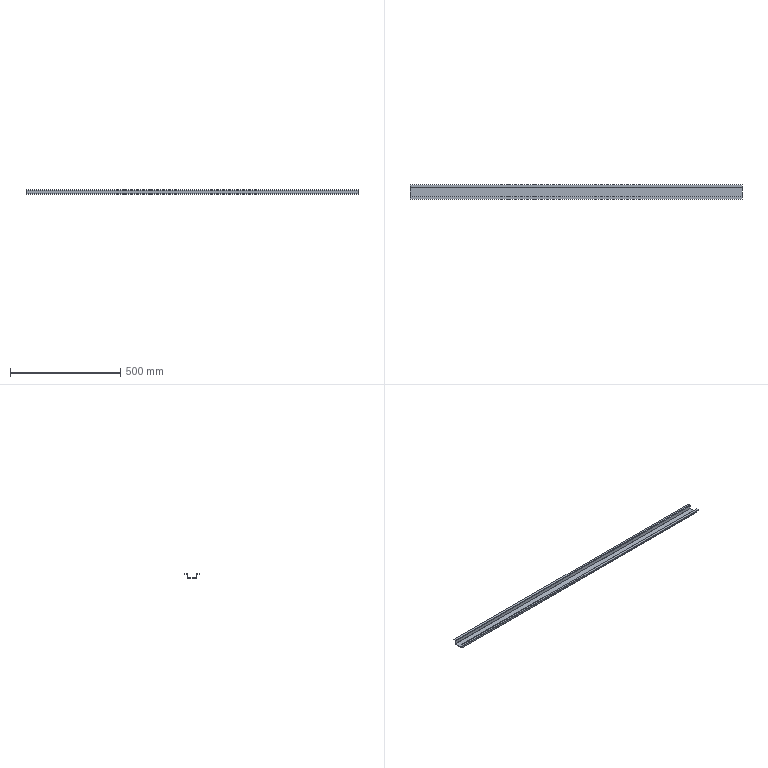Part | SolidWorks | features BaseBody 1 | 1 solid | 22 faces | box 1507 x 64 x 20 mm | volume 295191 mm3 | plane 14 | cylinder 8 | commonest cylinder face diameters 0.4 x4 4.4 x4
STEP:
#1=CARTESIAN_POINT('',(-730.,-22.2,-4.));
#2=VERTEX_POINT('',#1);
#3=CARTESIAN_POINT('',(-730.,-22.,-4.2));
#4=VERTEX_POINT('',#3);
#5=CARTESIAN_POINT('',(-730.,-22.2,-4.2));
#6=DIRECTION('',(-1.,0.,0.));
#7=DIRECTION('',(0.,0.,1.));
#8=AXIS2_PLACEMENT_3D('',#5,#6,#7);
#9=CIRCLE('',#8,0.2);
#10=EDGE_CURVE('',#2,#4,#9,.T.);
#11=ORIENTED_EDGE('',*,*,#10,.T.);
#12=CARTESIAN_POINT('',(777.,-22.,-4.2));
#13=VERTEX_POINT('',#12);
#14=CARTESIAN_POINT('',(777.,-22.,-4.2));
#15=DIRECTION('',(-1.,0.,0.));
#16=VECTOR('',#15,1000.);
#17=LINE('',#14,#16);
#18=EDGE_CURVE('',#13,#4,#17,.T.);
#19=ORIENTED_EDGE('',*,*,#18,.F.);
#20=CARTESIAN_POINT('',(777.,-22.2,-4.));
#21=VERTEX_POINT('',#20);
#22=CARTESIAN_POINT('',(777.,-22.2,-4.2));
#23=DIRECTION('',(1.,0.,0.));
#24=DIRECTION('',(0.,0.,1.));
#25=AXIS2_PLACEMENT_3D('',#22,#23,#24);
#26=CIRCLE('',#25,0.2);
#27=EDGE_CURVE('',#13,#21,#26,.T.);
#28=ORIENTED_EDGE('',*,*,#27,.T.);
#29=CARTESIAN_POINT('',(777.,-22.2,-4.));
#30=DIRECTION('',(1.,0.,0.));
#31=VECTOR('',#30,1000.);
#32=LINE('',#29,#31);
#33=EDGE_CURVE('',#2,#21,#32,.T.);
#34=ORIENTED_EDGE('',*,*,#33,.F.);
#35=EDGE_LOOP('',(#11,#19,#28,#34));
#36=FACE_OUTER_BOUND('',#35,.T.);
#37=CARTESIAN_POINT('',(2285.24,-22.2,-4.2));
#38=DIRECTION('',(-1.,0.,0.));
#39=DIRECTION('',(0.,0.,1.));
#40=AXIS2_PLACEMENT_3D('',#37,#38,#39);
#41=CYLINDRICAL_SURFACE('',#40,0.2);
#42=ADVANCED_FACE('',(#36),#41,.F.);
#43=CARTESIAN_POINT('',(-730.,-22.2,-2.));
#44=VERTEX_POINT('',#43);
#45=CARTESIAN_POINT('',(-730.,-20.,-4.2));
#46=VERTEX_POINT('',#45);
#47=CARTESIAN_POINT('',(-730.,-22.2,-4.2));
#48=DIRECTION('',(-1.,0.,0.));
#49=DIRECTION('',(0.,0.,1.));
#50=AXIS2_PLACEMENT_3D('',#47,#48,#49);
#51=CIRCLE('',#50,2.2);
#52=EDGE_CURVE('',#44,#46,#51,.T.);
#53=ORIENTED_EDGE('',*,*,#52,.F.);
#54=CARTESIAN_POINT('',(777.,-22.2,-2.));
#55=VERTEX_POINT('',#54);
#56=CARTESIAN_POINT('',(777.,-22.2,-2.));
#57=DIRECTION('',(1.,0.,0.));
#58=VECTOR('',#57,1000.);
#59=LINE('',#56,#58);
#60=EDGE_CURVE('',#44,#55,#59,.T.);
#61=ORIENTED_EDGE('',*,*,#60,.T.);
#62=CARTESIAN_POINT('',(777.,-20.,-4.2));
#63=VERTEX_POINT('',#62);
#64=CARTESIAN_POINT('',(777.,-22.2,-4.2));
#65=DIRECTION('',(1.,0.,0.));
#66=DIRECTION('',(0.,0.,1.));
#67=AXIS2_PLACEMENT_3D('',#64,#65,#66);
#68=CIRCLE('',#67,2.2);
#69=EDGE_CURVE('',#63,#55,#68,.T.);
#70=ORIENTED_EDGE('',*,*,#69,.F.);
#71=CARTESIAN_POINT('',(777.,-20.,-4.2));
#72=DIRECTION('',(-1.,0.,0.));
#73=VECTOR('',#72,1000.);
#74=LINE('',#71,#73);
#75=EDGE_CURVE('',#63,#46,#74,.T.);
#76=ORIENTED_EDGE('',*,*,#75,.T.);
#77=EDGE_LOOP('',(#53,#61,#70,#76));
#78=FACE_OUTER_BOUND('',#77,.T.);
#79=CARTESIAN_POINT('',(2285.24,-22.2,-4.2));
#80=DIRECTION('',(-1.,0.,0.));
#81=DIRECTION('',(0.,0.,1.));
#82=AXIS2_PLACEMENT_3D('',#79,#80,#81);
#83=CYLINDRICAL_SURFACE('',#82,2.2);
#84=ADVANCED_FACE('',(#78),#83,.T.);
#85=CARTESIAN_POINT('',(777.,22.2,-4.));
#86=VERTEX_POINT('',#85);
#87=CARTESIAN_POINT('',(777.,22.,-4.2));
#88=VERTEX_POINT('',#87);
#89=CARTESIAN_POINT('',(777.,22.2,-4.2));
#90=DIRECTION('',(1.,0.,0.));
#91=DIRECTION('',(0.,0.,-1.));
#92=AXIS2_PLACEMENT_3D('',#89,#90,#91);
#93=CIRCLE('',#92,0.2);
#94=EDGE_CURVE('',#86,#88,#93,.T.);
#95=ORIENTED_EDGE('',*,*,#94,.T.);
#96=CARTESIAN_POINT('',(-730.,22.,-4.2));
#97=VERTEX_POINT('',#96);
#98=CARTESIAN_POINT('',(-730.,22.,-4.2));
#99=DIRECTION('',(1.,0.,0.));
#100=VECTOR('',#99,1000.);
#101=LINE('',#98,#100);
#102=EDGE_CURVE('',#97,#88,#101,.T.);
#103=ORIENTED_EDGE('',*,*,#102,.F.);
#104=CARTESIAN_POINT('',(-730.,22.2,-4.));
#105=VERTEX_POINT('',#104);
#106=CARTESIAN_POINT('',(-730.,22.2,-4.2));
#107=DIRECTION('',(-1.,0.,0.));
#108=DIRECTION('',(0.,0.,-1.));
#109=AXIS2_PLACEMENT_3D('',#106,#107,#108);
#110=CIRCLE('',#109,0.2);
#111=EDGE_CURVE('',#97,#105,#110,.T.);
#112=ORIENTED_EDGE('',*,*,#111,.T.);
#113=CARTESIAN_POINT('',(-730.,22.2,-4.));
#114=DIRECTION('',(-1.,0.,0.));
#115=VECTOR('',#114,1000.);
#116=LINE('',#113,#115);
#117=EDGE_CURVE('',#86,#105,#116,.T.);
#118=ORIENTED_EDGE('',*,*,#117,.F.);
#119=EDGE_LOOP('',(#95,#103,#112,#118));
#120=FACE_OUTER_BOUND('',#119,.T.);
#121=CARTESIAN_POINT('',(-2237.915,22.2,-4.2));
#122=DIRECTION('',(1.,0.,0.));
#123=DIRECTION('',(0.,0.,-1.));
#124=AXIS2_PLACEMENT_3D('',#121,#122,#123);
#125=CYLINDRICAL_SURFACE('',#124,0.2);
#126=ADVANCED_FACE('',(#120),#125,.F.);
#127=CARTESIAN_POINT('',(777.,22.2,-2.));
#128=VERTEX_POINT('',#127);
#129=CARTESIAN_POINT('',(777.,20.,-4.2));
#130=VERTEX_POINT('',#129);
#131=CARTESIAN_POINT('',(777.,22.2,-4.2));
#132=DIRECTION('',(1.,0.,0.));
#133=DIRECTION('',(0.,0.,-1.));
#134=AXIS2_PLACEMENT_3D('',#131,#132,#133);
#135=CIRCLE('',#134,2.2);
#136=EDGE_CURVE('',#128,#130,#135,.T.);
#137=ORIENTED_EDGE('',*,*,#136,.F.);
#138=CARTESIAN_POINT('',(-730.,22.2,-2.));
#139=VERTEX_POINT('',#138);
#140=CARTESIAN_POINT('',(-730.,22.2,-2.));
#141=DIRECTION('',(-1.,0.,0.));
#142=VECTOR('',#141,1000.);
#143=LINE('',#140,#142);
#144=EDGE_CURVE('',#128,#139,#143,.T.);
#145=ORIENTED_EDGE('',*,*,#144,.T.);
#146=CARTESIAN_POINT('',(-730.,20.,-4.2));
#147=VERTEX_POINT('',#146);
#148=CARTESIAN_POINT('',(-730.,22.2,-4.2));
#149=DIRECTION('',(-1.,0.,0.));
#150=DIRECTION('',(0.,0.,-1.));
#151=AXIS2_PLACEMENT_3D('',#148,#149,#150);
#152=CIRCLE('',#151,2.2);
#153=EDGE_CURVE('',#147,#139,#152,.T.);
#154=ORIENTED_EDGE('',*,*,#153,.F.);
#155=CARTESIAN_POINT('',(-730.,20.,-4.2));
#156=DIRECTION('',(1.,0.,0.));
#157=VECTOR('',#156,1000.);
#158=LINE('',#155,#157);
#159=EDGE_CURVE('',#147,#130,#158,.T.);
#160=ORIENTED_EDGE('',*,*,#159,.T.);
#161=EDGE_LOOP('',(#137,#145,#154,#160));
#162=FACE_OUTER_BOUND('',#161,.T.);
#163=CARTESIAN_POINT('',(-2237.915,22.2,-4.2));
#164=DIRECTION('',(1.,0.,0.));
#165=DIRECTION('',(0.,0.,-1.));
#166=AXIS2_PLACEMENT_3D('',#163,#164,#165);
#167=CYLINDRICAL_SURFACE('',#166,2.2);
#168=ADVANCED_FACE('',(#162),#167,.T.);
#169=CARTESIAN_POINT('',(777.,20.,-19.8));
#170=VERTEX_POINT('',#169);
#171=CARTESIAN_POINT('',(777.,19.8,-20.));
#172=VERTEX_POINT('',#171);
#173=CARTESIAN_POINT('',(777.,19.8,-19.8));
#174=DIRECTION('',(-1.,0.,0.));
#175=DIRECTION('',(0.,0.,1.));
#176=AXIS2_PLACEMENT_3D('',#173,#174,#175);
#177=CIRCLE('',#176,0.2);
#178=EDGE_CURVE('',#170,#172,#177,.T.);
#179=ORIENTED_EDGE('',*,*,#178,.F.);
#180=CARTESIAN_POINT('',(-730.,20.,-19.8));
#181=VERTEX_POINT('',#180);
#182=CARTESIAN_POINT('',(777.,20.,-19.8));
#183=DIRECTION('',(-1.,0.,0.));
#184=VECTOR('',#183,1000.);
#185=LINE('',#182,#184);
#186=EDGE_CURVE('',#170,#181,#185,.T.);
#187=ORIENTED_EDGE('',*,*,#186,.T.);
#188=CARTESIAN_POINT('',(-730.,19.8,-20.));
#189=VERTEX_POINT('',#188);
#190=CARTESIAN_POINT('',(-730.,19.8,-19.8));
#191=DIRECTION('',(1.,0.,0.));
#192=DIRECTION('',(0.,0.,1.));
#193=AXIS2_PLACEMENT_3D('',#190,#191,#192);
#194=CIRCLE('',#193,0.2);
#195=EDGE_CURVE('',#189,#181,#194,.T.);
#196=ORIENTED_EDGE('',*,*,#195,.F.);
#197=CARTESIAN_POINT('',(777.,19.8,-20.));
#198=DIRECTION('',(-1.,0.,0.));
#199=VECTOR('',#198,1000.);
#200=LINE('',#197,#199);
#201=EDGE_CURVE('',#172,#189,#200,.T.);
#202=ORIENTED_EDGE('',*,*,#201,.F.);
#203=EDGE_LOOP('',(#179,#187,#196,#202));
#204=FACE_OUTER_BOUND('',#203,.T.);
#205=CARTESIAN_POINT('',(2285.87,19.8,-19.8));
#206=DIRECTION('',(-1.,0.,0.));
#207=DIRECTION('',(0.,0.,1.));
#208=AXIS2_PLACEMENT_3D('',#205,#206,#207);
#209=CYLINDRICAL_SURFACE('',#208,0.2);
#210=ADVANCED_FACE('',(#204),#209,.F.);
#211=CARTESIAN_POINT('',(777.,22.,-19.8));
#212=VERTEX_POINT('',#211);
#213=CARTESIAN_POINT('',(777.,19.8,-22.));
#214=VERTEX_POINT('',#213);
#215=CARTESIAN_POINT('',(777.,19.8,-19.8));
#216=DIRECTION('',(-1.,0.,0.));
#217=DIRECTION('',(0.,0.,1.));
#218=AXIS2_PLACEMENT_3D('',#215,#216,#217);
#219=CIRCLE('',#218,2.2);
#220=EDGE_CURVE('',#212,#214,#219,.T.);
#221=ORIENTED_EDGE('',*,*,#220,.T.);
#222=CARTESIAN_POINT('',(-730.,19.8,-22.));
#223=VERTEX_POINT('',#222);
#224=CARTESIAN_POINT('',(777.,19.8,-22.));
#225=DIRECTION('',(-1.,0.,0.));
#226=VECTOR('',#225,1000.);
#227=LINE('',#224,#226);
#228=EDGE_CURVE('',#214,#223,#227,.T.);
#229=ORIENTED_EDGE('',*,*,#228,.T.);
#230=CARTESIAN_POINT('',(-730.,22.,-19.8));
#231=VERTEX_POINT('',#230);
#232=CARTESIAN_POINT('',(-730.,19.8,-19.8));
#233=DIRECTION('',(1.,0.,0.));
#234=DIRECTION('',(0.,0.,1.));
#235=AXIS2_PLACEMENT_3D('',#232,#233,#234);
#236=CIRCLE('',#235,2.2);
#237=EDGE_CURVE('',#223,#231,#236,.T.);
#238=ORIENTED_EDGE('',*,*,#237,.T.);
#239=CARTESIAN_POINT('',(777.,22.,-19.8));
#240=DIRECTION('',(-1.,0.,0.));
#241=VECTOR('',#240,1000.);
#242=LINE('',#239,#241);
#243=EDGE_CURVE('',#212,#231,#242,.T.);
#244=ORIENTED_EDGE('',*,*,#243,.F.);
#245=EDGE_LOOP('',(#221,#229,#238,#244));
#246=FACE_OUTER_BOUND('',#245,.T.);
#247=CARTESIAN_POINT('',(2285.87,19.8,-19.8));
#248=DIRECTION('',(-1.,0.,0.));
#249=DIRECTION('',(0.,0.,1.));
#250=AXIS2_PLACEMENT_3D('',#247,#248,#249);
#251=CYLINDRICAL_SURFACE('',#250,2.2);
#252=ADVANCED_FACE('',(#246),#251,.T.);
#253=CARTESIAN_POINT('',(-730.,-20.,-19.8));
#254=VERTEX_POINT('',#253);
#255=CARTESIAN_POINT('',(-730.,-19.8,-20.));
#256=VERTEX_POINT('',#255);
#257=CARTESIAN_POINT('',(-730.,-19.8,-19.8));
#258=DIRECTION('',(1.,0.,0.));
#259=DIRECTION('',(0.,0.,-1.));
#260=AXIS2_PLACEMENT_3D('',#257,#258,#259);
#261=CIRCLE('',#260,0.2);
#262=EDGE_CURVE('',#254,#256,#261,.T.);
#263=ORIENTED_EDGE('',*,*,#262,.F.);
#264=CARTESIAN_POINT('',(777.,-20.,-19.8));
#265=VERTEX_POINT('',#264);
#266=CARTESIAN_POINT('',(-730.,-20.,-19.8));
#267=DIRECTION('',(1.,0.,0.));
#268=VECTOR('',#267,1000.);
#269=LINE('',#266,#268);
#270=EDGE_CURVE('',#254,#265,#269,.T.);
#271=ORIENTED_EDGE('',*,*,#270,.T.);
#272=CARTESIAN_POINT('',(777.,-19.8,-20.));
#273=VERTEX_POINT('',#272);
#274=CARTESIAN_POINT('',(777.,-19.8,-19.8));
#275=DIRECTION('',(-1.,0.,0.));
#276=DIRECTION('',(0.,0.,-1.));
#277=AXIS2_PLACEMENT_3D('',#274,#275,#276);
#278=CIRCLE('',#277,0.2);
#279=EDGE_CURVE('',#273,#265,#278,.T.);
#280=ORIENTED_EDGE('',*,*,#279,.F.);
#281=CARTESIAN_POINT('',(-730.,-19.8,-20.));
#282=DIRECTION('',(1.,0.,0.));
#283=VECTOR('',#282,1000.);
#284=LINE('',#281,#283);
#285=EDGE_CURVE('',#256,#273,#284,.T.);
#286=ORIENTED_EDGE('',*,*,#285,.F.);
#287=EDGE_LOOP('',(#263,#271,#280,#286));
#288=FACE_OUTER_BOUND('',#287,.T.);
#289=CARTESIAN_POINT('',(-2239.98,-19.8,-19.8));
#290=DIRECTION('',(1.,0.,0.));
#291=DIRECTION('',(0.,0.,-1.));
#292=AXIS2_PLACEMENT_3D('',#289,#290,#291);
#293=CYLINDRICAL_SURFACE('',#292,0.2);
#294=ADVANCED_FACE('',(#288),#293,.F.);
#295=CARTESIAN_POINT('',(-730.,-22.,-19.8));
#296=VERTEX_POINT('',#295);
#297=CARTESIAN_POINT('',(-730.,-19.8,-22.));
#298=VERTEX_POINT('',#297);
#299=CARTESIAN_POINT('',(-730.,-19.8,-19.8));
#300=DIRECTION('',(1.,0.,0.));
#301=DIRECTION('',(0.,0.,-1.));
#302=AXIS2_PLACEMENT_3D('',#299,#300,#301);
#303=CIRCLE('',#302,2.2);
#304=EDGE_CURVE('',#296,#298,#303,.T.);
#305=ORIENTED_EDGE('',*,*,#304,.T.);
#306=CARTESIAN_POINT('',(777.,-19.8,-22.));
#307=VERTEX_POINT('',#306);
#308=CARTESIAN_POINT('',(-730.,-19.8,-22.));
#309=DIRECTION('',(1.,0.,0.));
#310=VECTOR('',#309,1000.);
#311=LINE('',#308,#310);
#312=EDGE_CURVE('',#298,#307,#311,.T.);
#313=ORIENTED_EDGE('',*,*,#312,.T.);
#314=CARTESIAN_POINT('',(777.,-22.,-19.8));
#315=VERTEX_POINT('',#314);
#316=CARTESIAN_POINT('',(777.,-19.8,-19.8));
#317=DIRECTION('',(-1.,0.,0.));
#318=DIRECTION('',(0.,0.,-1.));
#319=AXIS2_PLACEMENT_3D('',#316,#317,#318);
#320=CIRCLE('',#319,2.2);
#321=EDGE_CURVE('',#307,#315,#320,.T.);
#322=ORIENTED_EDGE('',*,*,#321,.T.);
#323=CARTESIAN_POINT('',(-730.,-22.,-19.8));
#324=DIRECTION('',(1.,0.,0.));
#325=VECTOR('',#324,1000.);
#326=LINE('',#323,#325);
#327=EDGE_CURVE('',#296,#315,#326,.T.);
#328=ORIENTED_EDGE('',*,*,#327,.F.);
#329=EDGE_LOOP('',(#305,#313,#322,#328));
#330=FACE_OUTER_BOUND('',#329,.T.);
#331=CARTESIAN_POINT('',(-2239.98,-19.8,-19.8));
#332=DIRECTION('',(1.,0.,0.));
#333=DIRECTION('',(0.,0.,-1.));
#334=AXIS2_PLACEMENT_3D('',#331,#332,#333);
#335=CYLINDRICAL_SURFACE('',#334,2.2);
#336=ADVANCED_FACE('',(#330),#335,.T.);
#337=ORIENTED_EDGE('',*,*,#228,.F.);
#338=CARTESIAN_POINT('',(777.,20.,-22.));
#339=DIRECTION('',(0.,-1.,0.));
#340=VECTOR('',#339,1000.);
#341=LINE('',#338,#340);
#342=EDGE_CURVE('',#214,#307,#341,.T.);
#343=ORIENTED_EDGE('',*,*,#342,.T.);
#344=ORIENTED_EDGE('',*,*,#312,.F.);
#345=CARTESIAN_POINT('',(-730.,20.,-22.));
#346=DIRECTION('',(0.,-1.,0.));
#347=VECTOR('',#346,1000.);
#348=LINE('',#345,#347);
#349=EDGE_CURVE('',#223,#298,#348,.T.);
#350=ORIENTED_EDGE('',*,*,#349,.F.);
#351=EDGE_LOOP('',(#337,#343,#344,#350));
#352=FACE_OUTER_BOUND('',#351,.T.);
#353=CARTESIAN_POINT('',(-740.,20.,-22.));
#354=DIRECTION('',(0.,0.,1.));
#355=DIRECTION('',(1.,0.,0.));
#356=AXIS2_PLACEMENT_3D('',#353,#354,#355);
#357=PLANE('',#356);
#358=ADVANCED_FACE('',(#352),#357,.F.);
#359=CARTESIAN_POINT('',(777.,20.,-20.));
#360=DIRECTION('',(0.,-1.,0.));
#361=VECTOR('',#360,1000.);
#362=LINE('',#359,#361);
#363=EDGE_CURVE('',#172,#273,#362,.T.);
#364=ORIENTED_EDGE('',*,*,#363,.F.);
#365=ORIENTED_EDGE('',*,*,#201,.T.);
#366=CARTESIAN_POINT('',(-730.,20.,-20.));
#367=DIRECTION('',(0.,-1.,0.));
#368=VECTOR('',#367,1000.);
#369=LINE('',#366,#368);
#370=EDGE_CURVE('',#189,#256,#369,.T.);
#371=ORIENTED_EDGE('',*,*,#370,.T.);
#372=ORIENTED_EDGE('',*,*,#285,.T.);
#373=EDGE_LOOP('',(#364,#365,#371,#372));
#374=FACE_OUTER_BOUND('',#373,.T.);
#375=CARTESIAN_POINT('',(-740.,20.,-20.));
#376=DIRECTION('',(0.,0.,1.));
#377=DIRECTION('',(1.,0.,0.));
#378=AXIS2_PLACEMENT_3D('',#375,#376,#377);
#379=PLANE('',#378);
#380=ADVANCED_FACE('',(#374),#379,.T.);
#381=ORIENTED_EDGE('',*,*,#75,.F.);
#382=CARTESIAN_POINT('',(777.,-20.,-20.));
#383=DIRECTION('',(0.,0.,1.));
#384=VECTOR('',#383,1000.);
#385=LINE('',#382,#384);
#386=EDGE_CURVE('',#265,#63,#385,.T.);
#387=ORIENTED_EDGE('',*,*,#386,.F.);
#388=ORIENTED_EDGE('',*,*,#270,.F.);
#389=CARTESIAN_POINT('',(-730.,-20.,-20.));
#390=DIRECTION('',(0.,0.,1.));
#391=VECTOR('',#390,1000.);
#392=LINE('',#389,#391);
#393=EDGE_CURVE('',#254,#46,#392,.T.);
#394=ORIENTED_EDGE('',*,*,#393,.T.);
#395=EDGE_LOOP('',(#381,#387,#388,#394));
#396=FACE_OUTER_BOUND('',#395,.T.);
#397=CARTESIAN_POINT('',(-740.,-20.,-20.));
#398=DIRECTION('',(0.,1.,0.));
#399=DIRECTION('',(0.,0.,-1.));
#400=AXIS2_PLACEMENT_3D('',#397,#398,#399);
#401=PLANE('',#400);
#402=ADVANCED_FACE('',(#396),#401,.T.);
#403=CARTESIAN_POINT('',(777.,-22.,-20.));
#404=DIRECTION('',(0.,0.,1.));
#405=VECTOR('',#404,1000.);
#406=LINE('',#403,#405);
#407=EDGE_CURVE('',#315,#13,#406,.T.);
#408=ORIENTED_EDGE('',*,*,#407,.T.);
#409=ORIENTED_EDGE('',*,*,#18,.T.);
#410=CARTESIAN_POINT('',(-730.,-22.,-20.));
#411=DIRECTION('',(0.,0.,1.));
#412=VECTOR('',#411,1000.);
#413=LINE('',#410,#412);
#414=EDGE_CURVE('',#296,#4,#413,.T.);
#415=ORIENTED_EDGE('',*,*,#414,.F.);
#416=ORIENTED_EDGE('',*,*,#327,.T.);
#417=EDGE_LOOP('',(#408,#409,#415,#416));
#418=FACE_OUTER_BOUND('',#417,.T.);
#419=CARTESIAN_POINT('',(-740.,-22.,-20.));
#420=DIRECTION('',(0.,1.,0.));
#421=DIRECTION('',(0.,0.,-1.));
#422=AXIS2_PLACEMENT_3D('',#419,#420,#421);
#423=PLANE('',#422);
#424=ADVANCED_FACE('',(#418),#423,.F.);
#425=ORIENTED_EDGE('',*,*,#159,.F.);
#426=CARTESIAN_POINT('',(-730.,20.,-20.));
#427=DIRECTION('',(0.,0.,-1.));
#428=VECTOR('',#427,1000.);
#429=LINE('',#426,#428);
#430=EDGE_CURVE('',#147,#181,#429,.T.);
#431=ORIENTED_EDGE('',*,*,#430,.T.);
#432=ORIENTED_EDGE('',*,*,#186,.F.);
#433=CARTESIAN_POINT('',(777.,20.,-20.));
#434=DIRECTION('',(0.,0.,-1.));
#435=VECTOR('',#434,1000.);
#436=LINE('',#433,#435);
#437=EDGE_CURVE('',#130,#170,#436,.T.);
#438=ORIENTED_EDGE('',*,*,#437,.F.);
#439=EDGE_LOOP('',(#425,#431,#432,#438));
#440=FACE_OUTER_BOUND('',#439,.T.);
#441=CARTESIAN_POINT('',(-740.,20.,-20.));
#442=DIRECTION('',(0.,-1.,0.));
#443=DIRECTION('',(-1.,0.,0.));
#444=AXIS2_PLACEMENT_3D('',#441,#442,#443);
#445=PLANE('',#444);
#446=ADVANCED_FACE('',(#440),#445,.T.);
#447=CARTESIAN_POINT('',(-730.,22.,-20.));
#448=DIRECTION('',(0.,0.,-1.));
#449=VECTOR('',#448,1000.);
#450=LINE('',#447,#449);
#451=EDGE_CURVE('',#97,#231,#450,.T.);
#452=ORIENTED_EDGE('',*,*,#451,.F.);
#453=ORIENTED_EDGE('',*,*,#102,.T.);
#454=CARTESIAN_POINT('',(777.,22.,-20.));
#455=DIRECTION('',(0.,0.,-1.));
#456=VECTOR('',#455,1000.);
#457=LINE('',#454,#456);
#458=EDGE_CURVE('',#88,#212,#457,.T.);
#459=ORIENTED_EDGE('',*,*,#458,.T.);
#460=ORIENTED_EDGE('',*,*,#243,.T.);
#461=EDGE_LOOP('',(#452,#453,#459,#460));
#462=FACE_OUTER_BOUND('',#461,.T.);
#463=CARTESIAN_POINT('',(-740.,22.,-20.));
#464=DIRECTION('',(0.,-1.,0.));
#465=DIRECTION('',(-1.,0.,0.));
#466=AXIS2_PLACEMENT_3D('',#463,#464,#465);
#467=PLANE('',#466);
#468=ADVANCED_FACE('',(#462),#467,.F.);
#469=CARTESIAN_POINT('',(777.,32.,-4.));
#470=VERTEX_POINT('',#469);
#471=CARTESIAN_POINT('',(777.,20.,-4.));
#472=DIRECTION('',(0.,-1.,0.));
#473=VECTOR('',#472,1000.);
#474=LINE('',#471,#473);
#475=EDGE_CURVE('',#470,#86,#474,.T.);
#476=ORIENTED_EDGE('',*,*,#475,.T.);
#477=ORIENTED_EDGE('',*,*,#117,.T.);
#478=CARTESIAN_POINT('',(-730.,32.,-4.));
#479=VERTEX_POINT('',#478);
#480=CARTESIAN_POINT('',(-730.,20.,-4.));
#481=DIRECTION('',(0.,-1.,0.));
#482=VECTOR('',#481,1000.);
#483=LINE('',#480,#482);
#484=EDGE_CURVE('',#479,#105,#483,.T.);
#485=ORIENTED_EDGE('',*,*,#484,.F.);
#486=CARTESIAN_POINT('',(-740.,32.,-4.));
#487=DIRECTION('',(1.,0.,0.));
#488=VECTOR('',#487,1000.);
#489=LINE('',#486,#488);
#490=EDGE_CURVE('',#479,#470,#489,.T.);
#491=ORIENTED_EDGE('',*,*,#490,.T.);
#492=EDGE_LOOP('',(#476,#477,#485,#491));
#493=FACE_OUTER_BOUND('',#492,.T.);
#494=CARTESIAN_POINT('',(-740.,20.,-4.));
#495=DIRECTION('',(0.,0.,1.));
#496=DIRECTION('',(1.,0.,0.));
#497=AXIS2_PLACEMENT_3D('',#494,#495,#496);
#498=PLANE('',#497);
#499=ADVANCED_FACE('',(#493),#498,.F.);
#500=ORIENTED_EDGE('',*,*,#144,.F.);
#501=CARTESIAN_POINT('',(777.,32.,-2.));
#502=VERTEX_POINT('',#501);
#503=CARTESIAN_POINT('',(777.,20.,-2.));
#504=DIRECTION('',(0.,-1.,0.));
#505=VECTOR('',#504,1000.);
#506=LINE('',#503,#505);
#507=EDGE_CURVE('',#502,#128,#506,.T.);
#508=ORIENTED_EDGE('',*,*,#507,.F.);
#509=CARTESIAN_POINT('',(-730.,32.,-2.));
#510=VERTEX_POINT('',#509);
#511=CARTESIAN_POINT('',(-740.,32.,-2.));
#512=DIRECTION('',(1.,0.,0.));
#513=VECTOR('',#512,1000.);
#514=LINE('',#511,#513);
#515=EDGE_CURVE('',#510,#502,#514,.T.);
#516=ORIENTED_EDGE('',*,*,#515,.F.);
#517=CARTESIAN_POINT('',(-730.,20.,-2.));
#518=DIRECTION('',(0.,-1.,0.));
#519=VECTOR('',#518,1000.);
#520=LINE('',#517,#519);
#521=EDGE_CURVE('',#510,#139,#520,.T.);
#522=ORIENTED_EDGE('',*,*,#521,.T.);
#523=EDGE_LOOP('',(#500,#508,#516,#522));
#524=FACE_OUTER_BOUND('',#523,.T.);
#525=CARTESIAN_POINT('',(-740.,20.,-2.));
#526=DIRECTION('',(0.,0.,1.));
#527=DIRECTION('',(1.,0.,0.));
#528=AXIS2_PLACEMENT_3D('',#525,#526,#527);
#529=PLANE('',#528);
#530=ADVANCED_FACE('',(#524),#529,.T.);
#531=ORIENTED_EDGE('',*,*,#515,.T.);
#532=CARTESIAN_POINT('',(777.,32.,-3016.064));
#533=DIRECTION('',(0.,0.,1.));
#534=VECTOR('',#533,1000.);
#535=LINE('',#532,#534);
#536=EDGE_CURVE('',#470,#502,#535,.T.);
#537=ORIENTED_EDGE('',*,*,#536,.F.);
#538=ORIENTED_EDGE('',*,*,#490,.F.);
#539=CARTESIAN_POINT('',(-730.,32.,-3016.064));
#540=DIRECTION('',(0.,0.,1.));
#541=VECTOR('',#540,1000.);
#542=LINE('',#539,#541);
#543=EDGE_CURVE('',#479,#510,#542,.T.);
#544=ORIENTED_EDGE('',*,*,#543,.T.);
#545=EDGE_LOOP('',(#531,#537,#538,#544));
#546=FACE_OUTER_BOUND('',#545,.T.);
#547=CARTESIAN_POINT('',(-740.,32.,-3016.064));
#548=DIRECTION('',(0.,-1.,0.));
#549=DIRECTION('',(0.,0.,-1.));
#550=AXIS2_PLACEMENT_3D('',#547,#548,#549);
#551=PLANE('',#550);
#552=ADVANCED_FACE('',(#546),#551,.F.);
#553=CARTESIAN_POINT('',(-730.,-32.,-4.));
#554=VERTEX_POINT('',#553);
#555=CARTESIAN_POINT('',(-730.,-20.,-4.));
#556=DIRECTION('',(0.,1.,0.));
#557=VECTOR('',#556,1000.);
#558=LINE('',#555,#557);
#559=EDGE_CURVE('',#554,#2,#558,.T.);
#560=ORIENTED_EDGE('',*,*,#559,.T.);
#561=ORIENTED_EDGE('',*,*,#33,.T.);
#562=CARTESIAN_POINT('',(777.,-32.,-4.));
#563=VERTEX_POINT('',#562);
#564=CARTESIAN_POINT('',(777.,-20.,-4.));
#565=DIRECTION('',(0.,-1.,0.));
#566=VECTOR('',#565,1000.);
#567=LINE('',#564,#566);
#568=EDGE_CURVE('',#21,#563,#567,.T.);
#569=ORIENTED_EDGE('',*,*,#568,.T.);
#570=CARTESIAN_POINT('',(-740.,-32.,-4.));
#571=DIRECTION('',(1.,0.,0.));
#572=VECTOR('',#571,1000.);
#573=LINE('',#570,#572);
#574=EDGE_CURVE('',#554,#563,#573,.T.);
#575=ORIENTED_EDGE('',*,*,#574,.F.);
#576=EDGE_LOOP('',(#560,#561,#569,#575));
#577=FACE_OUTER_BOUND('',#576,.T.);
#578=CARTESIAN_POINT('',(-740.,-20.,-4.));
#579=DIRECTION('',(0.,0.,1.));
#580=DIRECTION('',(1.,0.,0.));
#581=AXIS2_PLACEMENT_3D('',#578,#579,#580);
#582=PLANE('',#581);
#583=ADVANCED_FACE('',(#577),#582,.F.);
#584=CARTESIAN_POINT('',(-730.,-32.,-2.));
#585=VERTEX_POINT('',#584);
#586=CARTESIAN_POINT('',(-730.,-32.,-3016.064));
#587=DIRECTION('',(0.,0.,1.));
#588=VECTOR('',#587,1000.);
#589=LINE('',#586,#588);
#590=EDGE_CURVE('',#554,#585,#589,.T.);
#591=ORIENTED_EDGE('',*,*,#590,.T.);
#592=CARTESIAN_POINT('',(-730.,-20.,-2.));
#593=DIRECTION('',(0.,1.,0.));
#594=VECTOR('',#593,1000.);
#595=LINE('',#592,#594);
#596=EDGE_CURVE('',#585,#44,#595,.T.);
#597=ORIENTED_EDGE('',*,*,#596,.T.);
#598=ORIENTED_EDGE('',*,*,#52,.T.);
#599=ORIENTED_EDGE('',*,*,#393,.F.);
#600=ORIENTED_EDGE('',*,*,#262,.T.);
#601=ORIENTED_EDGE('',*,*,#370,.F.);
#602=ORIENTED_EDGE('',*,*,#195,.T.);
#603=ORIENTED_EDGE('',*,*,#430,.F.);
#604=ORIENTED_EDGE('',*,*,#153,.T.);
#605=ORIENTED_EDGE('',*,*,#521,.F.);
#606=ORIENTED_EDGE('',*,*,#543,.F.);
#607=ORIENTED_EDGE('',*,*,#484,.T.);
#608=ORIENTED_EDGE('',*,*,#111,.F.);
#609=ORIENTED_EDGE('',*,*,#451,.T.);
#610=ORIENTED_EDGE('',*,*,#237,.F.);
#611=ORIENTED_EDGE('',*,*,#349,.T.);
#612=ORIENTED_EDGE('',*,*,#304,.F.);
#613=ORIENTED_EDGE('',*,*,#414,.T.);
#614=ORIENTED_EDGE('',*,*,#10,.F.);
#615=ORIENTED_EDGE('',*,*,#559,.F.);
#616=EDGE_LOOP('',(#591,#597,#598,#599,#600,#601,#602,#603,#604,#605,#606,#607,#608,#609,#610,#611,#612,#613,#614,#615));
#617=FACE_OUTER_BOUND('',#616,.T.);
#618=CARTESIAN_POINT('',(-730.,-20.,-3016.064));
#619=DIRECTION('',(-1.,0.,0.));
#620=DIRECTION('',(0.,0.,1.));
#621=AXIS2_PLACEMENT_3D('',#618,#619,#620);
#622=PLANE('',#621);
#623=ADVANCED_FACE('',(#617),#622,.T.);
#624=ORIENTED_EDGE('',*,*,#60,.F.);
#625=ORIENTED_EDGE('',*,*,#596,.F.);
#626=CARTESIAN_POINT('',(777.,-32.,-2.));
#627=VERTEX_POINT('',#626);
#628=CARTESIAN_POINT('',(-740.,-32.,-2.));
#629=DIRECTION('',(1.,0.,0.));
#630=VECTOR('',#629,1000.);
#631=LINE('',#628,#630);
#632=EDGE_CURVE('',#585,#627,#631,.T.);
#633=ORIENTED_EDGE('',*,*,#632,.T.);
#634=CARTESIAN_POINT('',(777.,-20.,-2.));
#635=DIRECTION('',(0.,-1.,0.));
#636=VECTOR('',#635,1000.);
#637=LINE('',#634,#636);
#638=EDGE_CURVE('',#55,#627,#637,.T.);
#639=ORIENTED_EDGE('',*,*,#638,.F.);
#640=EDGE_LOOP('',(#624,#625,#633,#639));
#641=FACE_OUTER_BOUND('',#640,.T.);
#642=CARTESIAN_POINT('',(-740.,-20.,-2.));
#643=DIRECTION('',(0.,0.,1.));
#644=DIRECTION('',(1.,0.,0.));
#645=AXIS2_PLACEMENT_3D('',#642,#643,#644);
#646=PLANE('',#645);
#647=ADVANCED_FACE('',(#641),#646,.T.);
#648=ORIENTED_EDGE('',*,*,#638,.T.);
#649=CARTESIAN_POINT('',(777.,-32.,-3016.064));
#650=DIRECTION('',(0.,0.,1.));
#651=VECTOR('',#650,1000.);
#652=LINE('',#649,#651);
#653=EDGE_CURVE('',#563,#627,#652,.T.);
#654=ORIENTED_EDGE('',*,*,#653,.F.);
#655=ORIENTED_EDGE('',*,*,#568,.F.);
#656=ORIENTED_EDGE('',*,*,#27,.F.);
#657=ORIENTED_EDGE('',*,*,#407,.F.);
#658=ORIENTED_EDGE('',*,*,#321,.F.);
#659=ORIENTED_EDGE('',*,*,#342,.F.);
#660=ORIENTED_EDGE('',*,*,#220,.F.);
#661=ORIENTED_EDGE('',*,*,#458,.F.);
#662=ORIENTED_EDGE('',*,*,#94,.F.);
#663=ORIENTED_EDGE('',*,*,#475,.F.);
#664=ORIENTED_EDGE('',*,*,#536,.T.);
#665=ORIENTED_EDGE('',*,*,#507,.T.);
#666=ORIENTED_EDGE('',*,*,#136,.T.);
#667=ORIENTED_EDGE('',*,*,#437,.T.);
#668=ORIENTED_EDGE('',*,*,#178,.T.);
#669=ORIENTED_EDGE('',*,*,#363,.T.);
#670=ORIENTED_EDGE('',*,*,#279,.T.);
#671=ORIENTED_EDGE('',*,*,#386,.T.);
#672=ORIENTED_EDGE('',*,*,#69,.T.);
#673=EDGE_LOOP('',(#648,#654,#655,#656,#657,#658,#659,#660,#661,#662,#663,#664,#665,#666,#667,#668,#669,#670,#671,#672));
#674=FACE_OUTER_BOUND('',#673,.T.);
#675=CARTESIAN_POINT('',(777.,-20.,-3016.064));
#676=DIRECTION('',(-1.,0.,0.));
#677=DIRECTION('',(0.,0.,1.));
#678=AXIS2_PLACEMENT_3D('',#675,#676,#677);
#679=PLANE('',#678);
#680=ADVANCED_FACE('',(#674),#679,.F.);
#681=ORIENTED_EDGE('',*,*,#653,.T.);
#682=ORIENTED_EDGE('',*,*,#632,.F.);
#683=ORIENTED_EDGE('',*,*,#590,.F.);
#684=ORIENTED_EDGE('',*,*,#574,.T.);
#685=EDGE_LOOP('',(#681,#682,#683,#684));
#686=FACE_OUTER_BOUND('',#685,.T.);
#687=CARTESIAN_POINT('',(-740.,-32.,-3016.064));
#688=DIRECTION('',(0.,-1.,0.));
#689=DIRECTION('',(-1.,0.,0.));
#690=AXIS2_PLACEMENT_3D('',#687,#688,#689);
#691=PLANE('',#690);
#692=ADVANCED_FACE('',(#686),#691,.T.);
#693=CLOSED_SHELL('',(#42,#84,#126,#168,#210,#252,#294,#336,#358,#380,#402,#424,#446,#468,#499,#530,#552,#583,#623,#647,#680,#692));
#694=MANIFOLD_SOLID_BREP('',#693);
#695=CARTESIAN_POINT('',(0.,0.,0.));
#696=DIRECTION('',(0.,0.,1.));
#697=DIRECTION('',(1.,0.,0.));
#698=AXIS2_PLACEMENT_3D('',#695,#696,#697);
#699=(LENGTH_UNIT()NAMED_UNIT(*)SI_UNIT(.MILLI.,.METRE.));
#700=UNCERTAINTY_MEASURE_WITH_UNIT(LENGTH_MEASURE(0.00001),#699,'','');
#701=(NAMED_UNIT(*)PLANE_ANGLE_UNIT()SI_UNIT($,.RADIAN.));
#702=(NAMED_UNIT(*)SI_UNIT($,.STERADIAN.)SOLID_ANGLE_UNIT());
#703=(GEOMETRIC_REPRESENTATION_CONTEXT(3)GLOBAL_UNCERTAINTY_ASSIGNED_CONTEXT((#700))GLOBAL_UNIT_ASSIGNED_CONTEXT((#699,#701,#702))REPRESENTATION_CONTEXT('',''));
#704=ADVANCED_BREP_SHAPE_REPRESENTATION('',(#694,#698),#703);